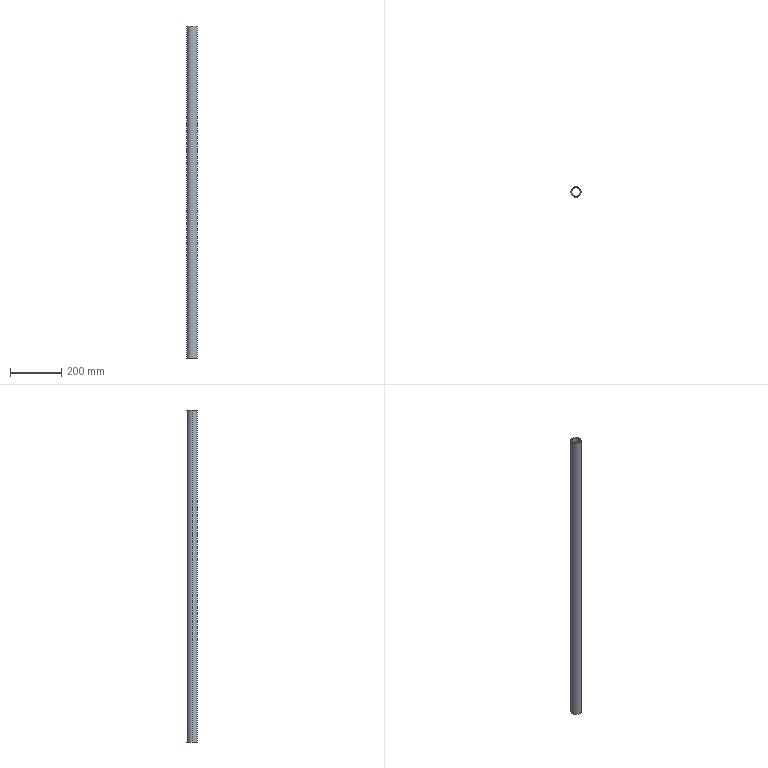Part | SolidWorks | features Extrusion 1 | 1 solid | 6 faces | box 40 x 40 x 1300 mm | volume 453332 mm3 | cylinder 4 | plane 2 | commonest cylinder face diameters 34 x2 40 x2
STEP:
#1=CARTESIAN_POINT('',(-17.,0.,650.));
#2=VERTEX_POINT('',#1);
#3=CARTESIAN_POINT('',(17.,0.,650.));
#4=VERTEX_POINT('',#3);
#5=CARTESIAN_POINT('',(0.,0.,650.));
#6=DIRECTION('',(0.,0.,1.));
#7=DIRECTION('',(1.,0.,0.));
#8=AXIS2_PLACEMENT_3D('',#5,#6,#7);
#9=CIRCLE('',#8,17.);
#10=EDGE_CURVE('',#2,#4,#9,.T.);
#11=ORIENTED_EDGE('',*,*,#10,.T.);
#12=CARTESIAN_POINT('',(17.,0.,-650.));
#13=VERTEX_POINT('',#12);
#14=CARTESIAN_POINT('',(17.,0.,650.));
#15=DIRECTION('',(0.,0.,-1.));
#16=VECTOR('',#15,1000.);
#17=LINE('',#14,#16);
#18=EDGE_CURVE('',#4,#13,#17,.T.);
#19=ORIENTED_EDGE('',*,*,#18,.T.);
#20=CARTESIAN_POINT('',(-17.,0.,-650.));
#21=VERTEX_POINT('',#20);
#22=CARTESIAN_POINT('',(0.,0.,-650.));
#23=DIRECTION('',(0.,0.,1.));
#24=DIRECTION('',(1.,0.,0.));
#25=AXIS2_PLACEMENT_3D('',#22,#23,#24);
#26=CIRCLE('',#25,17.);
#27=EDGE_CURVE('',#21,#13,#26,.T.);
#28=ORIENTED_EDGE('',*,*,#27,.F.);
#29=CARTESIAN_POINT('',(-17.,0.,650.));
#30=DIRECTION('',(0.,0.,-1.));
#31=VECTOR('',#30,1000.);
#32=LINE('',#29,#31);
#33=EDGE_CURVE('',#2,#21,#32,.T.);
#34=ORIENTED_EDGE('',*,*,#33,.F.);
#35=EDGE_LOOP('',(#11,#19,#28,#34));
#36=FACE_OUTER_BOUND('',#35,.T.);
#37=CARTESIAN_POINT('',(0.,0.,650.));
#38=DIRECTION('',(0.,0.,-1.));
#39=DIRECTION('',(-1.,0.,0.));
#40=AXIS2_PLACEMENT_3D('',#37,#38,#39);
#41=CYLINDRICAL_SURFACE('',#40,17.);
#42=ADVANCED_FACE('',(#36),#41,.F.);
#43=CARTESIAN_POINT('',(20.,0.,650.));
#44=VERTEX_POINT('',#43);
#45=CARTESIAN_POINT('',(-20.,0.,650.));
#46=VERTEX_POINT('',#45);
#47=CARTESIAN_POINT('',(0.,0.,650.));
#48=DIRECTION('',(0.,0.,1.));
#49=DIRECTION('',(1.,0.,0.));
#50=AXIS2_PLACEMENT_3D('',#47,#48,#49);
#51=CIRCLE('',#50,20.);
#52=EDGE_CURVE('',#44,#46,#51,.T.);
#53=ORIENTED_EDGE('',*,*,#52,.F.);
#54=CARTESIAN_POINT('',(20.,0.,-650.));
#55=VERTEX_POINT('',#54);
#56=CARTESIAN_POINT('',(20.,0.,650.));
#57=DIRECTION('',(0.,0.,-1.));
#58=VECTOR('',#57,1000.);
#59=LINE('',#56,#58);
#60=EDGE_CURVE('',#44,#55,#59,.T.);
#61=ORIENTED_EDGE('',*,*,#60,.T.);
#62=CARTESIAN_POINT('',(-20.,0.,-650.));
#63=VERTEX_POINT('',#62);
#64=CARTESIAN_POINT('',(0.,0.,-650.));
#65=DIRECTION('',(0.,0.,1.));
#66=DIRECTION('',(1.,0.,0.));
#67=AXIS2_PLACEMENT_3D('',#64,#65,#66);
#68=CIRCLE('',#67,20.);
#69=EDGE_CURVE('',#55,#63,#68,.T.);
#70=ORIENTED_EDGE('',*,*,#69,.T.);
#71=CARTESIAN_POINT('',(-20.,0.,650.));
#72=DIRECTION('',(0.,0.,-1.));
#73=VECTOR('',#72,1000.);
#74=LINE('',#71,#73);
#75=EDGE_CURVE('',#46,#63,#74,.T.);
#76=ORIENTED_EDGE('',*,*,#75,.F.);
#77=EDGE_LOOP('',(#53,#61,#70,#76));
#78=FACE_OUTER_BOUND('',#77,.T.);
#79=CARTESIAN_POINT('',(0.,0.,650.));
#80=DIRECTION('',(0.,0.,-1.));
#81=DIRECTION('',(-1.,0.,0.));
#82=AXIS2_PLACEMENT_3D('',#79,#80,#81);
#83=CYLINDRICAL_SURFACE('',#82,20.);
#84=ADVANCED_FACE('',(#78),#83,.T.);
#85=CARTESIAN_POINT('',(0.,0.,650.));
#86=DIRECTION('',(0.,0.,1.));
#87=DIRECTION('',(1.,0.,0.));
#88=AXIS2_PLACEMENT_3D('',#85,#86,#87);
#89=CIRCLE('',#88,20.);
#90=EDGE_CURVE('',#46,#44,#89,.T.);
#91=ORIENTED_EDGE('',*,*,#90,.T.);
#92=ORIENTED_EDGE('',*,*,#52,.T.);
#93=EDGE_LOOP('',(#91,#92));
#94=FACE_OUTER_BOUND('',#93,.T.);
#95=ORIENTED_EDGE('',*,*,#10,.F.);
#96=CARTESIAN_POINT('',(0.,0.,650.));
#97=DIRECTION('',(0.,0.,1.));
#98=DIRECTION('',(1.,0.,0.));
#99=AXIS2_PLACEMENT_3D('',#96,#97,#98);
#100=CIRCLE('',#99,17.);
#101=EDGE_CURVE('',#4,#2,#100,.T.);
#102=ORIENTED_EDGE('',*,*,#101,.F.);
#103=EDGE_LOOP('',(#95,#102));
#104=FACE_BOUND('',#103,.T.);
#105=CARTESIAN_POINT('',(0.,0.,650.));
#106=DIRECTION('',(0.,0.,1.));
#107=DIRECTION('',(1.,0.,0.));
#108=AXIS2_PLACEMENT_3D('',#105,#106,#107);
#109=PLANE('',#108);
#110=ADVANCED_FACE('',(#94,#104),#109,.T.);
#111=CARTESIAN_POINT('',(0.,0.,-650.));
#112=DIRECTION('',(0.,0.,1.));
#113=DIRECTION('',(1.,0.,0.));
#114=AXIS2_PLACEMENT_3D('',#111,#112,#113);
#115=CIRCLE('',#114,20.);
#116=EDGE_CURVE('',#63,#55,#115,.T.);
#117=ORIENTED_EDGE('',*,*,#116,.F.);
#118=ORIENTED_EDGE('',*,*,#69,.F.);
#119=EDGE_LOOP('',(#117,#118));
#120=FACE_OUTER_BOUND('',#119,.T.);
#121=ORIENTED_EDGE('',*,*,#27,.T.);
#122=CARTESIAN_POINT('',(0.,0.,-650.));
#123=DIRECTION('',(0.,0.,1.));
#124=DIRECTION('',(1.,0.,0.));
#125=AXIS2_PLACEMENT_3D('',#122,#123,#124);
#126=CIRCLE('',#125,17.);
#127=EDGE_CURVE('',#13,#21,#126,.T.);
#128=ORIENTED_EDGE('',*,*,#127,.T.);
#129=EDGE_LOOP('',(#121,#128));
#130=FACE_BOUND('',#129,.T.);
#131=CARTESIAN_POINT('',(0.,0.,-650.));
#132=DIRECTION('',(0.,0.,1.));
#133=DIRECTION('',(1.,0.,0.));
#134=AXIS2_PLACEMENT_3D('',#131,#132,#133);
#135=PLANE('',#134);
#136=ADVANCED_FACE('',(#120,#130),#135,.F.);
#137=ORIENTED_EDGE('',*,*,#60,.F.);
#138=ORIENTED_EDGE('',*,*,#90,.F.);
#139=ORIENTED_EDGE('',*,*,#75,.T.);
#140=ORIENTED_EDGE('',*,*,#116,.T.);
#141=EDGE_LOOP('',(#137,#138,#139,#140));
#142=FACE_OUTER_BOUND('',#141,.T.);
#143=CARTESIAN_POINT('',(0.,0.,650.));
#144=DIRECTION('',(0.,0.,-1.));
#145=DIRECTION('',(-1.,0.,0.));
#146=AXIS2_PLACEMENT_3D('',#143,#144,#145);
#147=CYLINDRICAL_SURFACE('',#146,20.);
#148=ADVANCED_FACE('',(#142),#147,.T.);
#149=ORIENTED_EDGE('',*,*,#18,.F.);
#150=ORIENTED_EDGE('',*,*,#101,.T.);
#151=ORIENTED_EDGE('',*,*,#33,.T.);
#152=ORIENTED_EDGE('',*,*,#127,.F.);
#153=EDGE_LOOP('',(#149,#150,#151,#152));
#154=FACE_OUTER_BOUND('',#153,.T.);
#155=CARTESIAN_POINT('',(0.,0.,650.));
#156=DIRECTION('',(0.,0.,-1.));
#157=DIRECTION('',(-1.,0.,0.));
#158=AXIS2_PLACEMENT_3D('',#155,#156,#157);
#159=CYLINDRICAL_SURFACE('',#158,17.);
#160=ADVANCED_FACE('',(#154),#159,.F.);
#161=CLOSED_SHELL('',(#42,#84,#110,#136,#148,#160));
#162=MANIFOLD_SOLID_BREP('',#161);
#163=CARTESIAN_POINT('',(0.,0.,0.));
#164=DIRECTION('',(0.,0.,1.));
#165=DIRECTION('',(1.,0.,0.));
#166=AXIS2_PLACEMENT_3D('',#163,#164,#165);
#167=(LENGTH_UNIT()NAMED_UNIT(*)SI_UNIT(.MILLI.,.METRE.));
#168=UNCERTAINTY_MEASURE_WITH_UNIT(LENGTH_MEASURE(0.00001),#167,'','');
#169=(NAMED_UNIT(*)PLANE_ANGLE_UNIT()SI_UNIT($,.RADIAN.));
#170=(NAMED_UNIT(*)SI_UNIT($,.STERADIAN.)SOLID_ANGLE_UNIT());
#171=(GEOMETRIC_REPRESENTATION_CONTEXT(3)GLOBAL_UNCERTAINTY_ASSIGNED_CONTEXT((#168))GLOBAL_UNIT_ASSIGNED_CONTEXT((#167,#169,#170))REPRESENTATION_CONTEXT('',''));
#172=ADVANCED_BREP_SHAPE_REPRESENTATION('',(#162,#166),#171);